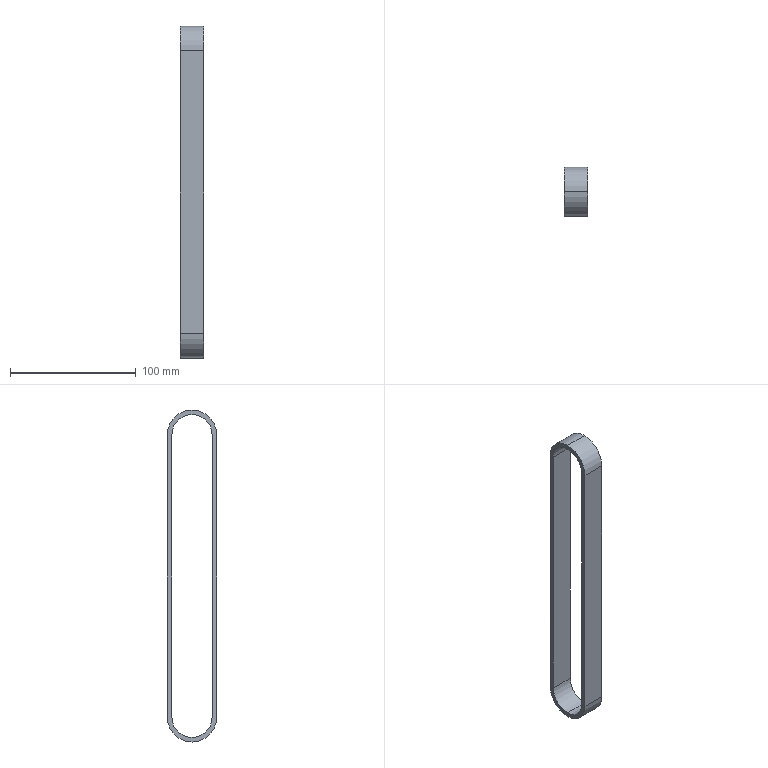Part | STEP file | TBN225L075 | 1 solid | 14 faces | box 19.05 x 39.218 x 264.218 mm | volume 38535 mm3 | cylinder 8 | plane 6 | commonest cylinder face diameters 32.018 x4 39.218 x4
STEP:
#1=CARTESIAN_POINT('',(9.525,0.,16.009));
#2=VERTEX_POINT('',#1);
#3=CARTESIAN_POINT('',(9.525,16.009,0.));
#4=VERTEX_POINT('',#3);
#5=CARTESIAN_POINT('',(9.525,0.,0.));
#6=DIRECTION('',(-1.,0.,0.));
#7=DIRECTION('',(0.,0.,1.));
#8=AXIS2_PLACEMENT_3D('',#5,#6,#7);
#9=CIRCLE('',#8,16.009);
#10=EDGE_CURVE('',#2,#4,#9,.T.);
#11=ORIENTED_EDGE('',*,*,#10,.F.);
#12=CARTESIAN_POINT('',(-9.525,0.,16.009));
#13=VERTEX_POINT('',#12);
#14=CARTESIAN_POINT('',(0.,0.,16.009));
#15=DIRECTION('',(-1.,0.,0.));
#16=VECTOR('',#15,1000.);
#17=LINE('',#14,#16);
#18=EDGE_CURVE('',#2,#13,#17,.T.);
#19=ORIENTED_EDGE('',*,*,#18,.T.);
#20=CARTESIAN_POINT('',(-9.525,16.009,0.));
#21=VERTEX_POINT('',#20);
#22=CARTESIAN_POINT('',(-9.525,0.,0.));
#23=DIRECTION('',(-1.,0.,0.));
#24=DIRECTION('',(0.,0.,1.));
#25=AXIS2_PLACEMENT_3D('',#22,#23,#24);
#26=CIRCLE('',#25,16.009);
#27=EDGE_CURVE('',#13,#21,#26,.T.);
#28=ORIENTED_EDGE('',*,*,#27,.T.);
#29=CARTESIAN_POINT('',(-9.525,16.009,0.));
#30=CARTESIAN_POINT('',(-3.175,16.009,0.));
#31=CARTESIAN_POINT('',(3.175,16.009,0.));
#32=CARTESIAN_POINT('',(9.525,16.009,0.));
#33=B_SPLINE_CURVE_WITH_KNOTS('',3,(#29,#30,#31,#32),.UNSPECIFIED.,.F.,.F.,(4,4),(0.,1.),.UNSPECIFIED.);
#34=EDGE_CURVE('',#21,#4,#33,.T.);
#35=ORIENTED_EDGE('',*,*,#34,.T.);
#36=EDGE_LOOP('',(#11,#19,#28,#35));
#37=FACE_OUTER_BOUND('',#36,.T.);
#38=CARTESIAN_POINT('',(0.,0.,0.));
#39=DIRECTION('',(-1.,0.,0.));
#40=DIRECTION('',(0.,0.,1.));
#41=AXIS2_PLACEMENT_3D('',#38,#39,#40);
#42=CYLINDRICAL_SURFACE('',#41,16.009);
#43=ADVANCED_FACE('',(#37),#42,.F.);
#44=CARTESIAN_POINT('',(9.525,-19.609,0.));
#45=VERTEX_POINT('',#44);
#46=CARTESIAN_POINT('',(9.525,0.,19.609));
#47=VERTEX_POINT('',#46);
#48=CARTESIAN_POINT('',(9.525,0.,0.));
#49=DIRECTION('',(-1.,0.,0.));
#50=DIRECTION('',(0.,0.,1.));
#51=AXIS2_PLACEMENT_3D('',#48,#49,#50);
#52=CIRCLE('',#51,19.609);
#53=EDGE_CURVE('',#45,#47,#52,.T.);
#54=ORIENTED_EDGE('',*,*,#53,.T.);
#55=CARTESIAN_POINT('',(-9.525,0.,19.609));
#56=VERTEX_POINT('',#55);
#57=CARTESIAN_POINT('',(0.,0.,19.609));
#58=DIRECTION('',(-1.,0.,0.));
#59=VECTOR('',#58,1000.);
#60=LINE('',#57,#59);
#61=EDGE_CURVE('',#47,#56,#60,.T.);
#62=ORIENTED_EDGE('',*,*,#61,.T.);
#63=CARTESIAN_POINT('',(-9.525,-19.609,0.));
#64=VERTEX_POINT('',#63);
#65=CARTESIAN_POINT('',(-9.525,0.,0.));
#66=DIRECTION('',(-1.,0.,0.));
#67=DIRECTION('',(0.,0.,1.));
#68=AXIS2_PLACEMENT_3D('',#65,#66,#67);
#69=CIRCLE('',#68,19.609);
#70=EDGE_CURVE('',#64,#56,#69,.T.);
#71=ORIENTED_EDGE('',*,*,#70,.F.);
#72=CARTESIAN_POINT('',(-9.525,-19.609,0.));
#73=DIRECTION('',(-1.,0.,0.));
#74=VECTOR('',#73,1000.);
#75=LINE('',#72,#74);
#76=EDGE_CURVE('',#45,#64,#75,.T.);
#77=ORIENTED_EDGE('',*,*,#76,.F.);
#78=EDGE_LOOP('',(#54,#62,#71,#77));
#79=FACE_OUTER_BOUND('',#78,.T.);
#80=CARTESIAN_POINT('',(0.,0.,0.));
#81=DIRECTION('',(-1.,0.,0.));
#82=DIRECTION('',(0.,0.,1.));
#83=AXIS2_PLACEMENT_3D('',#80,#81,#82);
#84=CYLINDRICAL_SURFACE('',#83,19.609);
#85=ADVANCED_FACE('',(#79),#84,.T.);
#86=CARTESIAN_POINT('',(-9.525,-19.609,-225.));
#87=VERTEX_POINT('',#86);
#88=CARTESIAN_POINT('',(-9.525,0.,-244.609));
#89=VERTEX_POINT('',#88);
#90=CARTESIAN_POINT('',(-9.525,0.,-225.));
#91=DIRECTION('',(1.,0.,0.));
#92=DIRECTION('',(0.,0.,-1.));
#93=AXIS2_PLACEMENT_3D('',#90,#91,#92);
#94=CIRCLE('',#93,19.609);
#95=EDGE_CURVE('',#87,#89,#94,.T.);
#96=ORIENTED_EDGE('',*,*,#95,.T.);
#97=CARTESIAN_POINT('',(9.525,0.,-244.609));
#98=VERTEX_POINT('',#97);
#99=CARTESIAN_POINT('',(0.,0.,-244.609));
#100=DIRECTION('',(1.,0.,0.));
#101=VECTOR('',#100,1000.);
#102=LINE('',#99,#101);
#103=EDGE_CURVE('',#89,#98,#102,.T.);
#104=ORIENTED_EDGE('',*,*,#103,.T.);
#105=CARTESIAN_POINT('',(9.525,-19.609,-225.));
#106=VERTEX_POINT('',#105);
#107=CARTESIAN_POINT('',(9.525,0.,-225.));
#108=DIRECTION('',(1.,0.,0.));
#109=DIRECTION('',(0.,0.,-1.));
#110=AXIS2_PLACEMENT_3D('',#107,#108,#109);
#111=CIRCLE('',#110,19.609);
#112=EDGE_CURVE('',#106,#98,#111,.T.);
#113=ORIENTED_EDGE('',*,*,#112,.F.);
#114=CARTESIAN_POINT('',(-9.525,-19.609,-225.));
#115=DIRECTION('',(-1.,0.,0.));
#116=VECTOR('',#115,1000.);
#117=LINE('',#114,#116);
#118=EDGE_CURVE('',#106,#87,#117,.T.);
#119=ORIENTED_EDGE('',*,*,#118,.T.);
#120=EDGE_LOOP('',(#96,#104,#113,#119));
#121=FACE_OUTER_BOUND('',#120,.T.);
#122=CARTESIAN_POINT('',(0.,0.,-225.));
#123=DIRECTION('',(1.,0.,0.));
#124=DIRECTION('',(0.,0.,-1.));
#125=AXIS2_PLACEMENT_3D('',#122,#123,#124);
#126=CYLINDRICAL_SURFACE('',#125,19.609);
#127=ADVANCED_FACE('',(#121),#126,.T.);
#128=CARTESIAN_POINT('',(-9.525,0.,-241.009));
#129=VERTEX_POINT('',#128);
#130=CARTESIAN_POINT('',(-9.525,16.009,-225.));
#131=VERTEX_POINT('',#130);
#132=CARTESIAN_POINT('',(-9.525,0.,-225.));
#133=DIRECTION('',(1.,0.,0.));
#134=DIRECTION('',(0.,0.,-1.));
#135=AXIS2_PLACEMENT_3D('',#132,#133,#134);
#136=CIRCLE('',#135,16.009);
#137=EDGE_CURVE('',#129,#131,#136,.T.);
#138=ORIENTED_EDGE('',*,*,#137,.F.);
#139=CARTESIAN_POINT('',(9.525,0.,-241.009));
#140=VERTEX_POINT('',#139);
#141=CARTESIAN_POINT('',(0.,0.,-241.009));
#142=DIRECTION('',(1.,0.,0.));
#143=VECTOR('',#142,1000.);
#144=LINE('',#141,#143);
#145=EDGE_CURVE('',#129,#140,#144,.T.);
#146=ORIENTED_EDGE('',*,*,#145,.T.);
#147=CARTESIAN_POINT('',(9.525,16.009,-225.));
#148=VERTEX_POINT('',#147);
#149=CARTESIAN_POINT('',(9.525,0.,-225.));
#150=DIRECTION('',(1.,0.,0.));
#151=DIRECTION('',(0.,0.,-1.));
#152=AXIS2_PLACEMENT_3D('',#149,#150,#151);
#153=CIRCLE('',#152,16.009);
#154=EDGE_CURVE('',#140,#148,#153,.T.);
#155=ORIENTED_EDGE('',*,*,#154,.T.);
#156=CARTESIAN_POINT('',(9.525,16.009,-225.));
#157=DIRECTION('',(1.,0.,0.));
#158=VECTOR('',#157,1000.);
#159=LINE('',#156,#158);
#160=EDGE_CURVE('',#131,#148,#159,.T.);
#161=ORIENTED_EDGE('',*,*,#160,.F.);
#162=EDGE_LOOP('',(#138,#146,#155,#161));
#163=FACE_OUTER_BOUND('',#162,.T.);
#164=CARTESIAN_POINT('',(0.,0.,-225.));
#165=DIRECTION('',(1.,0.,0.));
#166=DIRECTION('',(0.,0.,-1.));
#167=AXIS2_PLACEMENT_3D('',#164,#165,#166);
#168=CYLINDRICAL_SURFACE('',#167,16.009);
#169=ADVANCED_FACE('',(#163),#168,.F.);
#170=ORIENTED_EDGE('',*,*,#160,.T.);
#171=CARTESIAN_POINT('',(9.525,16.009,-225.));
#172=DIRECTION('',(0.,0.,1.));
#173=VECTOR('',#172,1000.);
#174=LINE('',#171,#173);
#175=EDGE_CURVE('',#148,#4,#174,.T.);
#176=ORIENTED_EDGE('',*,*,#175,.T.);
#177=ORIENTED_EDGE('',*,*,#34,.F.);
#178=CARTESIAN_POINT('',(-9.525,16.009,-225.));
#179=DIRECTION('',(0.,0.,1.));
#180=VECTOR('',#179,1000.);
#181=LINE('',#178,#180);
#182=EDGE_CURVE('',#131,#21,#181,.T.);
#183=ORIENTED_EDGE('',*,*,#182,.F.);
#184=EDGE_LOOP('',(#170,#176,#177,#183));
#185=FACE_OUTER_BOUND('',#184,.T.);
#186=CARTESIAN_POINT('',(9.525,16.009,-225.));
#187=DIRECTION('',(0.,-1.,0.));
#188=DIRECTION('',(0.,0.,-1.));
#189=AXIS2_PLACEMENT_3D('',#186,#187,#188);
#190=PLANE('',#189);
#191=ADVANCED_FACE('',(#185),#190,.T.);
#192=CARTESIAN_POINT('',(9.525,19.609,-225.));
#193=VERTEX_POINT('',#192);
#194=CARTESIAN_POINT('',(-9.525,19.609,-225.));
#195=VERTEX_POINT('',#194);
#196=CARTESIAN_POINT('',(-9.525,19.609,-225.));
#197=DIRECTION('',(-1.,0.,0.));
#198=VECTOR('',#197,1000.);
#199=LINE('',#196,#198);
#200=EDGE_CURVE('',#193,#195,#199,.T.);
#201=ORIENTED_EDGE('',*,*,#200,.T.);
#202=CARTESIAN_POINT('',(-9.525,19.609,0.));
#203=VERTEX_POINT('',#202);
#204=CARTESIAN_POINT('',(-9.525,19.609,-225.));
#205=DIRECTION('',(0.,0.,1.));
#206=VECTOR('',#205,1000.);
#207=LINE('',#204,#206);
#208=EDGE_CURVE('',#195,#203,#207,.T.);
#209=ORIENTED_EDGE('',*,*,#208,.T.);
#210=CARTESIAN_POINT('',(9.525,19.609,0.));
#211=VERTEX_POINT('',#210);
#212=CARTESIAN_POINT('',(9.525,19.609,0.));
#213=CARTESIAN_POINT('',(3.175,19.609,0.));
#214=CARTESIAN_POINT('',(-3.175,19.609,0.));
#215=CARTESIAN_POINT('',(-9.525,19.609,0.));
#216=B_SPLINE_CURVE_WITH_KNOTS('',3,(#212,#213,#214,#215),.UNSPECIFIED.,.F.,.F.,(4,4),(0.,1.),.UNSPECIFIED.);
#217=EDGE_CURVE('',#211,#203,#216,.T.);
#218=ORIENTED_EDGE('',*,*,#217,.F.);
#219=CARTESIAN_POINT('',(9.525,19.609,-225.));
#220=DIRECTION('',(0.,0.,1.));
#221=VECTOR('',#220,1000.);
#222=LINE('',#219,#221);
#223=EDGE_CURVE('',#193,#211,#222,.T.);
#224=ORIENTED_EDGE('',*,*,#223,.F.);
#225=EDGE_LOOP('',(#201,#209,#218,#224));
#226=FACE_OUTER_BOUND('',#225,.T.);
#227=CARTESIAN_POINT('',(-9.525,19.609,-225.));
#228=DIRECTION('',(0.,1.,0.));
#229=DIRECTION('',(0.,0.,1.));
#230=AXIS2_PLACEMENT_3D('',#227,#228,#229);
#231=PLANE('',#230);
#232=ADVANCED_FACE('',(#226),#231,.T.);
#233=ORIENTED_EDGE('',*,*,#145,.F.);
#234=CARTESIAN_POINT('',(-9.525,-16.009,-225.));
#235=VERTEX_POINT('',#234);
#236=CARTESIAN_POINT('',(-9.525,0.,-225.));
#237=DIRECTION('',(1.,0.,0.));
#238=DIRECTION('',(0.,0.,-1.));
#239=AXIS2_PLACEMENT_3D('',#236,#237,#238);
#240=CIRCLE('',#239,16.009);
#241=EDGE_CURVE('',#235,#129,#240,.T.);
#242=ORIENTED_EDGE('',*,*,#241,.F.);
#243=CARTESIAN_POINT('',(9.525,-16.009,-225.));
#244=VERTEX_POINT('',#243);
#245=CARTESIAN_POINT('',(9.525,-16.009,-225.));
#246=DIRECTION('',(1.,0.,0.));
#247=VECTOR('',#246,1000.);
#248=LINE('',#245,#247);
#249=EDGE_CURVE('',#235,#244,#248,.T.);
#250=ORIENTED_EDGE('',*,*,#249,.T.);
#251=CARTESIAN_POINT('',(9.525,0.,-225.));
#252=DIRECTION('',(1.,0.,0.));
#253=DIRECTION('',(0.,0.,-1.));
#254=AXIS2_PLACEMENT_3D('',#251,#252,#253);
#255=CIRCLE('',#254,16.009);
#256=EDGE_CURVE('',#244,#140,#255,.T.);
#257=ORIENTED_EDGE('',*,*,#256,.T.);
#258=EDGE_LOOP('',(#233,#242,#250,#257));
#259=FACE_OUTER_BOUND('',#258,.T.);
#260=CARTESIAN_POINT('',(0.,0.,-225.));
#261=DIRECTION('',(1.,0.,0.));
#262=DIRECTION('',(0.,0.,-1.));
#263=AXIS2_PLACEMENT_3D('',#260,#261,#262);
#264=CYLINDRICAL_SURFACE('',#263,16.009);
#265=ADVANCED_FACE('',(#259),#264,.F.);
#266=ORIENTED_EDGE('',*,*,#103,.F.);
#267=CARTESIAN_POINT('',(-9.525,0.,-225.));
#268=DIRECTION('',(1.,0.,0.));
#269=DIRECTION('',(0.,0.,-1.));
#270=AXIS2_PLACEMENT_3D('',#267,#268,#269);
#271=CIRCLE('',#270,19.609);
#272=EDGE_CURVE('',#89,#195,#271,.T.);
#273=ORIENTED_EDGE('',*,*,#272,.T.);
#274=ORIENTED_EDGE('',*,*,#200,.F.);
#275=CARTESIAN_POINT('',(9.525,0.,-225.));
#276=DIRECTION('',(1.,0.,0.));
#277=DIRECTION('',(0.,0.,-1.));
#278=AXIS2_PLACEMENT_3D('',#275,#276,#277);
#279=CIRCLE('',#278,19.609);
#280=EDGE_CURVE('',#98,#193,#279,.T.);
#281=ORIENTED_EDGE('',*,*,#280,.F.);
#282=EDGE_LOOP('',(#266,#273,#274,#281));
#283=FACE_OUTER_BOUND('',#282,.T.);
#284=CARTESIAN_POINT('',(0.,0.,-225.));
#285=DIRECTION('',(1.,0.,0.));
#286=DIRECTION('',(0.,0.,-1.));
#287=AXIS2_PLACEMENT_3D('',#284,#285,#286);
#288=CYLINDRICAL_SURFACE('',#287,19.609);
#289=ADVANCED_FACE('',(#283),#288,.T.);
#290=CARTESIAN_POINT('',(-9.525,-16.009,0.));
#291=VERTEX_POINT('',#290);
#292=CARTESIAN_POINT('',(9.525,-16.009,0.));
#293=VERTEX_POINT('',#292);
#294=CARTESIAN_POINT('',(9.525,-16.009,0.));
#295=DIRECTION('',(1.,0.,0.));
#296=VECTOR('',#295,1000.);
#297=LINE('',#294,#296);
#298=EDGE_CURVE('',#291,#293,#297,.T.);
#299=ORIENTED_EDGE('',*,*,#298,.T.);
#300=CARTESIAN_POINT('',(9.525,-16.009,0.));
#301=DIRECTION('',(0.,0.,-1.));
#302=VECTOR('',#301,1000.);
#303=LINE('',#300,#302);
#304=EDGE_CURVE('',#293,#244,#303,.T.);
#305=ORIENTED_EDGE('',*,*,#304,.T.);
#306=ORIENTED_EDGE('',*,*,#249,.F.);
#307=CARTESIAN_POINT('',(-9.525,-16.009,0.));
#308=DIRECTION('',(0.,0.,-1.));
#309=VECTOR('',#308,1000.);
#310=LINE('',#307,#309);
#311=EDGE_CURVE('',#291,#235,#310,.T.);
#312=ORIENTED_EDGE('',*,*,#311,.F.);
#313=EDGE_LOOP('',(#299,#305,#306,#312));
#314=FACE_OUTER_BOUND('',#313,.T.);
#315=CARTESIAN_POINT('',(9.525,-16.009,0.));
#316=DIRECTION('',(0.,1.,0.));
#317=DIRECTION('',(0.,0.,1.));
#318=AXIS2_PLACEMENT_3D('',#315,#316,#317);
#319=PLANE('',#318);
#320=ADVANCED_FACE('',(#314),#319,.T.);
#321=ORIENTED_EDGE('',*,*,#76,.T.);
#322=CARTESIAN_POINT('',(-9.525,-19.609,0.));
#323=DIRECTION('',(0.,0.,-1.));
#324=VECTOR('',#323,1000.);
#325=LINE('',#322,#324);
#326=EDGE_CURVE('',#64,#87,#325,.T.);
#327=ORIENTED_EDGE('',*,*,#326,.T.);
#328=ORIENTED_EDGE('',*,*,#118,.F.);
#329=CARTESIAN_POINT('',(9.525,-19.609,0.));
#330=DIRECTION('',(0.,0.,-1.));
#331=VECTOR('',#330,1000.);
#332=LINE('',#329,#331);
#333=EDGE_CURVE('',#45,#106,#332,.T.);
#334=ORIENTED_EDGE('',*,*,#333,.F.);
#335=EDGE_LOOP('',(#321,#327,#328,#334));
#336=FACE_OUTER_BOUND('',#335,.T.);
#337=CARTESIAN_POINT('',(-9.525,-19.609,0.));
#338=DIRECTION('',(0.,-1.,0.));
#339=DIRECTION('',(0.,0.,-1.));
#340=AXIS2_PLACEMENT_3D('',#337,#338,#339);
#341=PLANE('',#340);
#342=ADVANCED_FACE('',(#336),#341,.T.);
#343=CARTESIAN_POINT('',(-9.525,0.,0.));
#344=DIRECTION('',(-1.,0.,0.));
#345=DIRECTION('',(0.,0.,1.));
#346=AXIS2_PLACEMENT_3D('',#343,#344,#345);
#347=CIRCLE('',#346,16.009);
#348=EDGE_CURVE('',#291,#13,#347,.T.);
#349=ORIENTED_EDGE('',*,*,#348,.F.);
#350=ORIENTED_EDGE('',*,*,#311,.T.);
#351=ORIENTED_EDGE('',*,*,#241,.T.);
#352=ORIENTED_EDGE('',*,*,#137,.T.);
#353=ORIENTED_EDGE('',*,*,#182,.T.);
#354=ORIENTED_EDGE('',*,*,#27,.F.);
#355=EDGE_LOOP('',(#349,#350,#351,#352,#353,#354));
#356=FACE_BOUND('',#355,.T.);
#357=ORIENTED_EDGE('',*,*,#70,.T.);
#358=CARTESIAN_POINT('',(-9.525,0.,0.));
#359=DIRECTION('',(-1.,0.,0.));
#360=DIRECTION('',(0.,0.,1.));
#361=AXIS2_PLACEMENT_3D('',#358,#359,#360);
#362=CIRCLE('',#361,19.609);
#363=EDGE_CURVE('',#56,#203,#362,.T.);
#364=ORIENTED_EDGE('',*,*,#363,.T.);
#365=ORIENTED_EDGE('',*,*,#208,.F.);
#366=ORIENTED_EDGE('',*,*,#272,.F.);
#367=ORIENTED_EDGE('',*,*,#95,.F.);
#368=ORIENTED_EDGE('',*,*,#326,.F.);
#369=EDGE_LOOP('',(#357,#364,#365,#366,#367,#368));
#370=FACE_OUTER_BOUND('',#369,.T.);
#371=CARTESIAN_POINT('',(-9.525,-16.009,0.));
#372=DIRECTION('',(1.,0.,0.));
#373=DIRECTION('',(0.,0.,-1.));
#374=AXIS2_PLACEMENT_3D('',#371,#372,#373);
#375=PLANE('',#374);
#376=ADVANCED_FACE('',(#356,#370),#375,.F.);
#377=ORIENTED_EDGE('',*,*,#61,.F.);
#378=CARTESIAN_POINT('',(9.525,0.,0.));
#379=DIRECTION('',(-1.,0.,0.));
#380=DIRECTION('',(0.,0.,1.));
#381=AXIS2_PLACEMENT_3D('',#378,#379,#380);
#382=CIRCLE('',#381,19.609);
#383=EDGE_CURVE('',#47,#211,#382,.T.);
#384=ORIENTED_EDGE('',*,*,#383,.T.);
#385=ORIENTED_EDGE('',*,*,#217,.T.);
#386=ORIENTED_EDGE('',*,*,#363,.F.);
#387=EDGE_LOOP('',(#377,#384,#385,#386));
#388=FACE_OUTER_BOUND('',#387,.T.);
#389=CARTESIAN_POINT('',(0.,0.,0.));
#390=DIRECTION('',(-1.,0.,0.));
#391=DIRECTION('',(0.,0.,1.));
#392=AXIS2_PLACEMENT_3D('',#389,#390,#391);
#393=CYLINDRICAL_SURFACE('',#392,19.609);
#394=ADVANCED_FACE('',(#388),#393,.T.);
#395=ORIENTED_EDGE('',*,*,#53,.F.);
#396=ORIENTED_EDGE('',*,*,#333,.T.);
#397=ORIENTED_EDGE('',*,*,#112,.T.);
#398=ORIENTED_EDGE('',*,*,#280,.T.);
#399=ORIENTED_EDGE('',*,*,#223,.T.);
#400=ORIENTED_EDGE('',*,*,#383,.F.);
#401=EDGE_LOOP('',(#395,#396,#397,#398,#399,#400));
#402=FACE_OUTER_BOUND('',#401,.T.);
#403=CARTESIAN_POINT('',(9.525,0.,0.));
#404=DIRECTION('',(-1.,0.,0.));
#405=DIRECTION('',(0.,0.,1.));
#406=AXIS2_PLACEMENT_3D('',#403,#404,#405);
#407=CIRCLE('',#406,16.009);
#408=EDGE_CURVE('',#293,#2,#407,.T.);
#409=ORIENTED_EDGE('',*,*,#408,.T.);
#410=ORIENTED_EDGE('',*,*,#10,.T.);
#411=ORIENTED_EDGE('',*,*,#175,.F.);
#412=ORIENTED_EDGE('',*,*,#154,.F.);
#413=ORIENTED_EDGE('',*,*,#256,.F.);
#414=ORIENTED_EDGE('',*,*,#304,.F.);
#415=EDGE_LOOP('',(#409,#410,#411,#412,#413,#414));
#416=FACE_BOUND('',#415,.T.);
#417=CARTESIAN_POINT('',(9.525,-19.609,0.));
#418=DIRECTION('',(-1.,0.,0.));
#419=DIRECTION('',(0.,0.,1.));
#420=AXIS2_PLACEMENT_3D('',#417,#418,#419);
#421=PLANE('',#420);
#422=ADVANCED_FACE('',(#402,#416),#421,.F.);
#423=ORIENTED_EDGE('',*,*,#18,.F.);
#424=ORIENTED_EDGE('',*,*,#408,.F.);
#425=ORIENTED_EDGE('',*,*,#298,.F.);
#426=ORIENTED_EDGE('',*,*,#348,.T.);
#427=EDGE_LOOP('',(#423,#424,#425,#426));
#428=FACE_OUTER_BOUND('',#427,.T.);
#429=CARTESIAN_POINT('',(0.,0.,0.));
#430=DIRECTION('',(-1.,0.,0.));
#431=DIRECTION('',(0.,0.,1.));
#432=AXIS2_PLACEMENT_3D('',#429,#430,#431);
#433=CYLINDRICAL_SURFACE('',#432,16.009);
#434=ADVANCED_FACE('',(#428),#433,.F.);
#435=CLOSED_SHELL('',(#43,#85,#127,#169,#191,#232,#265,#289,#320,#342,#376,#394,#422,#434));
#436=MANIFOLD_SOLID_BREP('',#435);
#437=CARTESIAN_POINT('',(0.,0.,0.));
#438=DIRECTION('',(0.,0.,1.));
#439=DIRECTION('',(1.,0.,0.));
#440=AXIS2_PLACEMENT_3D('',#437,#438,#439);
#441=(LENGTH_UNIT()NAMED_UNIT(*)SI_UNIT(.MILLI.,.METRE.));
#442=UNCERTAINTY_MEASURE_WITH_UNIT(LENGTH_MEASURE(0.00001),#441,'','');
#443=(NAMED_UNIT(*)PLANE_ANGLE_UNIT()SI_UNIT($,.RADIAN.));
#444=(NAMED_UNIT(*)SI_UNIT($,.STERADIAN.)SOLID_ANGLE_UNIT());
#445=(GEOMETRIC_REPRESENTATION_CONTEXT(3)GLOBAL_UNCERTAINTY_ASSIGNED_CONTEXT((#442))GLOBAL_UNIT_ASSIGNED_CONTEXT((#441,#443,#444))REPRESENTATION_CONTEXT('',''));
#446=ADVANCED_BREP_SHAPE_REPRESENTATION('',(#436,#440),#445);